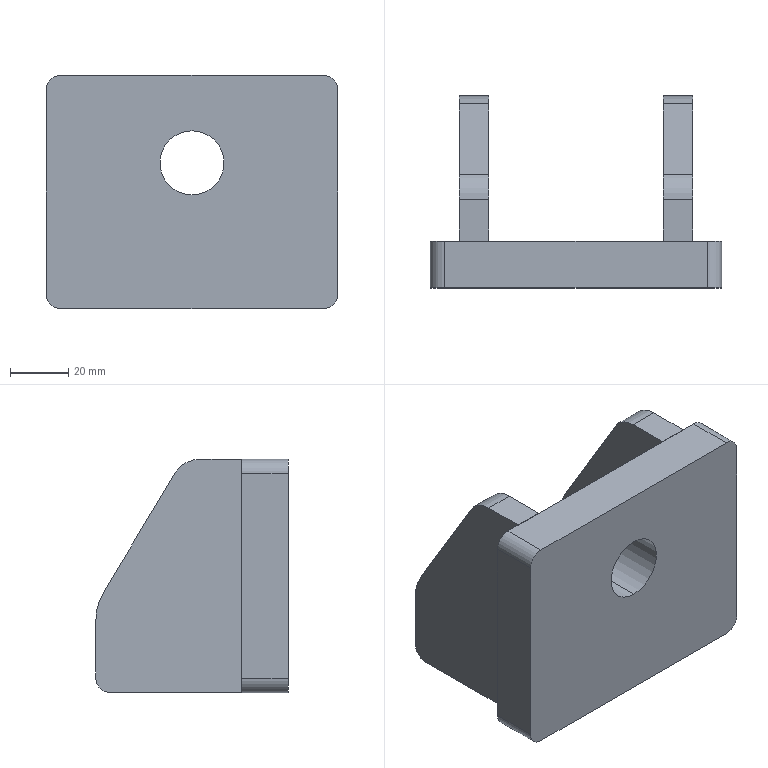Part | SolidWorks | features BaseBody 3 | 3 solids | 32 faces | box 100 x 66 x 80 mm | volume 186311 mm3 | plane 20 | cylinder 12 | commonest cylinder face diameters 10 x6 20 x2 22 x2 40 x2
STEP:
#1=CARTESIAN_POINT('',(30.,8.,30.));
#2=VERTEX_POINT('',#1);
#3=CARTESIAN_POINT('',(30.,8.,-50.));
#4=VERTEX_POINT('',#3);
#5=CARTESIAN_POINT('',(30.,8.,-50.));
#6=DIRECTION('',(0.,0.,-1.));
#7=VECTOR('',#6,1000.);
#8=LINE('',#5,#7);
#9=EDGE_CURVE('',#2,#4,#8,.T.);
#10=ORIENTED_EDGE('',*,*,#9,.T.);
#11=CARTESIAN_POINT('',(40.,8.,-50.));
#12=VERTEX_POINT('',#11);
#13=CARTESIAN_POINT('',(40.,8.,-50.));
#14=DIRECTION('',(-1.,0.,0.));
#15=VECTOR('',#14,1000.);
#16=LINE('',#13,#15);
#17=EDGE_CURVE('',#12,#4,#16,.T.);
#18=ORIENTED_EDGE('',*,*,#17,.F.);
#19=CARTESIAN_POINT('',(40.,8.,30.));
#20=VERTEX_POINT('',#19);
#21=CARTESIAN_POINT('',(40.,8.,-50.));
#22=DIRECTION('',(0.,0.,-1.));
#23=VECTOR('',#22,1000.);
#24=LINE('',#21,#23);
#25=EDGE_CURVE('',#20,#12,#24,.T.);
#26=ORIENTED_EDGE('',*,*,#25,.F.);
#27=CARTESIAN_POINT('',(40.,8.,30.));
#28=DIRECTION('',(-1.,0.,0.));
#29=VECTOR('',#28,1000.);
#30=LINE('',#27,#29);
#31=EDGE_CURVE('',#20,#2,#30,.T.);
#32=ORIENTED_EDGE('',*,*,#31,.T.);
#33=EDGE_LOOP('',(#10,#18,#26,#32));
#34=FACE_OUTER_BOUND('',#33,.T.);
#35=CARTESIAN_POINT('',(40.,8.,-50.));
#36=DIRECTION('',(0.,1.,0.));
#37=DIRECTION('',(0.,0.,1.));
#38=AXIS2_PLACEMENT_3D('',#35,#36,#37);
#39=PLANE('',#38);
#40=ADVANCED_FACE('',(#34),#39,.F.);
#41=CARTESIAN_POINT('',(30.,53.,-50.));
#42=VERTEX_POINT('',#41);
#43=CARTESIAN_POINT('',(30.,53.,-50.));
#44=DIRECTION('',(0.,1.,0.));
#45=VECTOR('',#44,1000.);
#46=LINE('',#43,#45);
#47=EDGE_CURVE('',#4,#42,#46,.T.);
#48=ORIENTED_EDGE('',*,*,#47,.T.);
#49=CARTESIAN_POINT('',(40.,53.,-50.));
#50=VERTEX_POINT('',#49);
#51=CARTESIAN_POINT('',(40.,53.,-50.));
#52=DIRECTION('',(-1.,0.,0.));
#53=VECTOR('',#52,1000.);
#54=LINE('',#51,#53);
#55=EDGE_CURVE('',#50,#42,#54,.T.);
#56=ORIENTED_EDGE('',*,*,#55,.F.);
#57=CARTESIAN_POINT('',(40.,53.,-50.));
#58=DIRECTION('',(0.,1.,0.));
#59=VECTOR('',#58,1000.);
#60=LINE('',#57,#59);
#61=EDGE_CURVE('',#12,#50,#60,.T.);
#62=ORIENTED_EDGE('',*,*,#61,.F.);
#63=ORIENTED_EDGE('',*,*,#17,.T.);
#64=EDGE_LOOP('',(#48,#56,#62,#63));
#65=FACE_OUTER_BOUND('',#64,.T.);
#66=CARTESIAN_POINT('',(40.,53.,-50.));
#67=DIRECTION('',(0.,0.,1.));
#68=DIRECTION('',(0.,-1.,0.));
#69=AXIS2_PLACEMENT_3D('',#66,#67,#68);
#70=PLANE('',#69);
#71=ADVANCED_FACE('',(#65),#70,.F.);
#72=CARTESIAN_POINT('',(30.,58.,-45.));
#73=VERTEX_POINT('',#72);
#74=CARTESIAN_POINT('',(30.,53.,-45.));
#75=DIRECTION('',(1.,0.,0.));
#76=DIRECTION('',(0.,0.,1.));
#77=AXIS2_PLACEMENT_3D('',#74,#75,#76);
#78=CIRCLE('',#77,5.);
#79=EDGE_CURVE('',#42,#73,#78,.T.);
#80=ORIENTED_EDGE('',*,*,#79,.T.);
#81=CARTESIAN_POINT('',(40.,58.,-45.));
#82=VERTEX_POINT('',#81);
#83=CARTESIAN_POINT('',(40.,58.,-45.));
#84=DIRECTION('',(-1.,0.,0.));
#85=VECTOR('',#84,1000.);
#86=LINE('',#83,#85);
#87=EDGE_CURVE('',#82,#73,#86,.T.);
#88=ORIENTED_EDGE('',*,*,#87,.F.);
#89=CARTESIAN_POINT('',(40.,53.,-45.));
#90=DIRECTION('',(1.,0.,0.));
#91=DIRECTION('',(0.,0.,1.));
#92=AXIS2_PLACEMENT_3D('',#89,#90,#91);
#93=CIRCLE('',#92,5.);
#94=EDGE_CURVE('',#50,#82,#93,.T.);
#95=ORIENTED_EDGE('',*,*,#94,.F.);
#96=ORIENTED_EDGE('',*,*,#55,.T.);
#97=EDGE_LOOP('',(#80,#88,#95,#96));
#98=FACE_OUTER_BOUND('',#97,.T.);
#99=CARTESIAN_POINT('',(40.,53.,-45.));
#100=DIRECTION('',(-1.,0.,0.));
#101=DIRECTION('',(0.,0.,1.));
#102=AXIS2_PLACEMENT_3D('',#99,#100,#101);
#103=CYLINDRICAL_SURFACE('',#102,5.);
#104=ADVANCED_FACE('',(#98),#103,.T.);
#105=CARTESIAN_POINT('',(30.,58.,-25.54));
#106=VERTEX_POINT('',#105);
#107=CARTESIAN_POINT('',(30.,58.,-25.54));
#108=DIRECTION('',(0.,0.,1.));
#109=VECTOR('',#108,1000.);
#110=LINE('',#107,#109);
#111=EDGE_CURVE('',#73,#106,#110,.T.);
#112=ORIENTED_EDGE('',*,*,#111,.T.);
#113=CARTESIAN_POINT('',(40.,58.,-25.54));
#114=VERTEX_POINT('',#113);
#115=CARTESIAN_POINT('',(40.,58.,-25.54));
#116=DIRECTION('',(-1.,0.,0.));
#117=VECTOR('',#116,1000.);
#118=LINE('',#115,#117);
#119=EDGE_CURVE('',#114,#106,#118,.T.);
#120=ORIENTED_EDGE('',*,*,#119,.F.);
#121=CARTESIAN_POINT('',(40.,58.,-25.54));
#122=DIRECTION('',(0.,0.,1.));
#123=VECTOR('',#122,1000.);
#124=LINE('',#121,#123);
#125=EDGE_CURVE('',#82,#114,#124,.T.);
#126=ORIENTED_EDGE('',*,*,#125,.F.);
#127=ORIENTED_EDGE('',*,*,#87,.T.);
#128=EDGE_LOOP('',(#112,#120,#126,#127));
#129=FACE_OUTER_BOUND('',#128,.T.);
#130=CARTESIAN_POINT('',(40.,58.,-25.54));
#131=DIRECTION('',(0.,-1.,0.));
#132=DIRECTION('',(0.,0.,-1.));
#133=AXIS2_PLACEMENT_3D('',#130,#131,#132);
#134=PLANE('',#133);
#135=ADVANCED_FACE('',(#129),#134,.F.);
#136=CARTESIAN_POINT('',(30.,55.15,-15.25));
#137=VERTEX_POINT('',#136);
#138=CARTESIAN_POINT('',(30.,38.,-25.54));
#139=DIRECTION('',(1.,0.,0.));
#140=DIRECTION('',(0.,0.,1.));
#141=AXIS2_PLACEMENT_3D('',#138,#139,#140);
#142=CIRCLE('',#141,20.);
#143=EDGE_CURVE('',#106,#137,#142,.T.);
#144=ORIENTED_EDGE('',*,*,#143,.T.);
#145=CARTESIAN_POINT('',(40.,55.15,-15.25));
#146=VERTEX_POINT('',#145);
#147=CARTESIAN_POINT('',(40.,55.15,-15.25));
#148=DIRECTION('',(-1.,0.,0.));
#149=VECTOR('',#148,1000.);
#150=LINE('',#147,#149);
#151=EDGE_CURVE('',#146,#137,#150,.T.);
#152=ORIENTED_EDGE('',*,*,#151,.F.);
#153=CARTESIAN_POINT('',(40.,38.,-25.54));
#154=DIRECTION('',(1.,0.,0.));
#155=DIRECTION('',(0.,0.,1.));
#156=AXIS2_PLACEMENT_3D('',#153,#154,#155);
#157=CIRCLE('',#156,20.);
#158=EDGE_CURVE('',#114,#146,#157,.T.);
#159=ORIENTED_EDGE('',*,*,#158,.F.);
#160=ORIENTED_EDGE('',*,*,#119,.T.);
#161=EDGE_LOOP('',(#144,#152,#159,#160));
#162=FACE_OUTER_BOUND('',#161,.T.);
#163=CARTESIAN_POINT('',(40.,38.,-25.54));
#164=DIRECTION('',(-1.,0.,0.));
#165=DIRECTION('',(0.,0.,1.));
#166=AXIS2_PLACEMENT_3D('',#163,#164,#165);
#167=CYLINDRICAL_SURFACE('',#166,20.);
#168=ADVANCED_FACE('',(#162),#167,.T.);
#169=CARTESIAN_POINT('',(30.,30.913,25.145));
#170=VERTEX_POINT('',#169);
#171=CARTESIAN_POINT('',(30.,30.913,25.145));
#172=DIRECTION('',(0.,-0.5145,0.8575));
#173=VECTOR('',#172,1000.);
#174=LINE('',#171,#173);
#175=EDGE_CURVE('',#137,#170,#174,.T.);
#176=ORIENTED_EDGE('',*,*,#175,.T.);
#177=CARTESIAN_POINT('',(40.,30.913,25.145));
#178=VERTEX_POINT('',#177);
#179=CARTESIAN_POINT('',(40.,30.913,25.145));
#180=DIRECTION('',(-1.,0.,0.));
#181=VECTOR('',#180,1000.);
#182=LINE('',#179,#181);
#183=EDGE_CURVE('',#178,#170,#182,.T.);
#184=ORIENTED_EDGE('',*,*,#183,.F.);
#185=CARTESIAN_POINT('',(40.,30.913,25.145));
#186=DIRECTION('',(0.,-0.5145,0.8575));
#187=VECTOR('',#186,1000.);
#188=LINE('',#185,#187);
#189=EDGE_CURVE('',#146,#178,#188,.T.);
#190=ORIENTED_EDGE('',*,*,#189,.F.);
#191=ORIENTED_EDGE('',*,*,#151,.T.);
#192=EDGE_LOOP('',(#176,#184,#190,#191));
#193=FACE_OUTER_BOUND('',#192,.T.);
#194=CARTESIAN_POINT('',(40.,30.913,25.145));
#195=DIRECTION('',(0.,-0.8575,-0.5145));
#196=DIRECTION('',(0.,0.5145,-0.8575));
#197=AXIS2_PLACEMENT_3D('',#194,#195,#196);
#198=PLANE('',#197);
#199=ADVANCED_FACE('',(#193),#198,.F.);
#200=CARTESIAN_POINT('',(30.,22.338,30.));
#201=VERTEX_POINT('',#200);
#202=CARTESIAN_POINT('',(30.,22.338,20.));
#203=DIRECTION('',(1.,0.,0.));
#204=DIRECTION('',(0.,0.,1.));
#205=AXIS2_PLACEMENT_3D('',#202,#203,#204);
#206=CIRCLE('',#205,10.);
#207=EDGE_CURVE('',#170,#201,#206,.T.);
#208=ORIENTED_EDGE('',*,*,#207,.T.);
#209=CARTESIAN_POINT('',(40.,22.338,30.));
#210=VERTEX_POINT('',#209);
#211=CARTESIAN_POINT('',(40.,22.338,30.));
#212=DIRECTION('',(-1.,0.,0.));
#213=VECTOR('',#212,1000.);
#214=LINE('',#211,#213);
#215=EDGE_CURVE('',#210,#201,#214,.T.);
#216=ORIENTED_EDGE('',*,*,#215,.F.);
#217=CARTESIAN_POINT('',(40.,22.338,20.));
#218=DIRECTION('',(1.,0.,0.));
#219=DIRECTION('',(0.,0.,1.));
#220=AXIS2_PLACEMENT_3D('',#217,#218,#219);
#221=CIRCLE('',#220,10.);
#222=EDGE_CURVE('',#178,#210,#221,.T.);
#223=ORIENTED_EDGE('',*,*,#222,.F.);
#224=ORIENTED_EDGE('',*,*,#183,.T.);
#225=EDGE_LOOP('',(#208,#216,#223,#224));
#226=FACE_OUTER_BOUND('',#225,.T.);
#227=CARTESIAN_POINT('',(40.,22.338,20.));
#228=DIRECTION('',(-1.,0.,0.));
#229=DIRECTION('',(0.,0.,1.));
#230=AXIS2_PLACEMENT_3D('',#227,#228,#229);
#231=CYLINDRICAL_SURFACE('',#230,10.);
#232=ADVANCED_FACE('',(#226),#231,.T.);
#233=CARTESIAN_POINT('',(30.,8.,30.));
#234=DIRECTION('',(0.,-1.,0.));
#235=VECTOR('',#234,1000.);
#236=LINE('',#233,#235);
#237=EDGE_CURVE('',#201,#2,#236,.T.);
#238=ORIENTED_EDGE('',*,*,#237,.T.);
#239=ORIENTED_EDGE('',*,*,#31,.F.);
#240=CARTESIAN_POINT('',(40.,8.,30.));
#241=DIRECTION('',(0.,-1.,0.));
#242=VECTOR('',#241,1000.);
#243=LINE('',#240,#242);
#244=EDGE_CURVE('',#210,#20,#243,.T.);
#245=ORIENTED_EDGE('',*,*,#244,.F.);
#246=ORIENTED_EDGE('',*,*,#215,.T.);
#247=EDGE_LOOP('',(#238,#239,#245,#246));
#248=FACE_OUTER_BOUND('',#247,.T.);
#249=CARTESIAN_POINT('',(40.,8.,30.));
#250=DIRECTION('',(0.,0.,-1.));
#251=DIRECTION('',(-1.,0.,0.));
#252=AXIS2_PLACEMENT_3D('',#249,#250,#251);
#253=PLANE('',#252);
#254=ADVANCED_FACE('',(#248),#253,.F.);
#255=ORIENTED_EDGE('',*,*,#25,.T.);
#256=ORIENTED_EDGE('',*,*,#61,.T.);
#257=ORIENTED_EDGE('',*,*,#94,.T.);
#258=ORIENTED_EDGE('',*,*,#125,.T.);
#259=ORIENTED_EDGE('',*,*,#158,.T.);
#260=ORIENTED_EDGE('',*,*,#189,.T.);
#261=ORIENTED_EDGE('',*,*,#222,.T.);
#262=ORIENTED_EDGE('',*,*,#244,.T.);
#263=EDGE_LOOP('',(#255,#256,#257,#258,#259,#260,#261,#262));
#264=FACE_OUTER_BOUND('',#263,.T.);
#265=CARTESIAN_POINT('',(40.,22.338,20.));
#266=DIRECTION('',(-1.,0.,0.));
#267=DIRECTION('',(0.,0.,1.));
#268=AXIS2_PLACEMENT_3D('',#265,#266,#267);
#269=PLANE('',#268);
#270=ADVANCED_FACE('',(#264),#269,.F.);
#271=ORIENTED_EDGE('',*,*,#9,.F.);
#272=ORIENTED_EDGE('',*,*,#237,.F.);
#273=ORIENTED_EDGE('',*,*,#207,.F.);
#274=ORIENTED_EDGE('',*,*,#175,.F.);
#275=ORIENTED_EDGE('',*,*,#143,.F.);
#276=ORIENTED_EDGE('',*,*,#111,.F.);
#277=ORIENTED_EDGE('',*,*,#79,.F.);
#278=ORIENTED_EDGE('',*,*,#47,.F.);
#279=EDGE_LOOP('',(#271,#272,#273,#274,#275,#276,#277,#278));
#280=FACE_OUTER_BOUND('',#279,.T.);
#281=CARTESIAN_POINT('',(30.,22.338,20.));
#282=DIRECTION('',(-1.,0.,0.));
#283=DIRECTION('',(0.,0.,1.));
#284=AXIS2_PLACEMENT_3D('',#281,#282,#283);
#285=PLANE('',#284);
#286=ADVANCED_FACE('',(#280),#285,.T.);
#287=CLOSED_SHELL('',(#40,#71,#104,#135,#168,#199,#232,#254,#270,#286));
#288=MANIFOLD_SOLID_BREP('',#287);
#289=CARTESIAN_POINT('',(-30.,8.,30.));
#290=VERTEX_POINT('',#289);
#291=CARTESIAN_POINT('',(-30.,8.,-50.));
#292=VERTEX_POINT('',#291);
#293=CARTESIAN_POINT('',(-30.,8.,-50.));
#294=DIRECTION('',(0.,0.,-1.));
#295=VECTOR('',#294,1000.);
#296=LINE('',#293,#295);
#297=EDGE_CURVE('',#290,#292,#296,.T.);
#298=ORIENTED_EDGE('',*,*,#297,.F.);
#299=CARTESIAN_POINT('',(-40.,8.,30.));
#300=VERTEX_POINT('',#299);
#301=CARTESIAN_POINT('',(-40.,8.,30.));
#302=DIRECTION('',(1.,0.,0.));
#303=VECTOR('',#302,1000.);
#304=LINE('',#301,#303);
#305=EDGE_CURVE('',#300,#290,#304,.T.);
#306=ORIENTED_EDGE('',*,*,#305,.F.);
#307=CARTESIAN_POINT('',(-40.,8.,-50.));
#308=VERTEX_POINT('',#307);
#309=CARTESIAN_POINT('',(-40.,8.,-50.));
#310=DIRECTION('',(0.,0.,-1.));
#311=VECTOR('',#310,1000.);
#312=LINE('',#309,#311);
#313=EDGE_CURVE('',#300,#308,#312,.T.);
#314=ORIENTED_EDGE('',*,*,#313,.T.);
#315=CARTESIAN_POINT('',(-40.,8.,-50.));
#316=DIRECTION('',(1.,0.,0.));
#317=VECTOR('',#316,1000.);
#318=LINE('',#315,#317);
#319=EDGE_CURVE('',#308,#292,#318,.T.);
#320=ORIENTED_EDGE('',*,*,#319,.T.);
#321=EDGE_LOOP('',(#298,#306,#314,#320));
#322=FACE_OUTER_BOUND('',#321,.T.);
#323=CARTESIAN_POINT('',(-40.,8.,-50.));
#324=DIRECTION('',(0.,1.,0.));
#325=DIRECTION('',(0.,0.,1.));
#326=AXIS2_PLACEMENT_3D('',#323,#324,#325);
#327=PLANE('',#326);
#328=ADVANCED_FACE('',(#322),#327,.F.);
#329=CARTESIAN_POINT('',(-30.,53.,-50.));
#330=VERTEX_POINT('',#329);
#331=CARTESIAN_POINT('',(-30.,53.,-50.));
#332=DIRECTION('',(0.,1.,0.));
#333=VECTOR('',#332,1000.);
#334=LINE('',#331,#333);
#335=EDGE_CURVE('',#292,#330,#334,.T.);
#336=ORIENTED_EDGE('',*,*,#335,.F.);
#337=ORIENTED_EDGE('',*,*,#319,.F.);
#338=CARTESIAN_POINT('',(-40.,53.,-50.));
#339=VERTEX_POINT('',#338);
#340=CARTESIAN_POINT('',(-40.,53.,-50.));
#341=DIRECTION('',(0.,1.,0.));
#342=VECTOR('',#341,1000.);
#343=LINE('',#340,#342);
#344=EDGE_CURVE('',#308,#339,#343,.T.);
#345=ORIENTED_EDGE('',*,*,#344,.T.);
#346=CARTESIAN_POINT('',(-40.,53.,-50.));
#347=DIRECTION('',(1.,0.,0.));
#348=VECTOR('',#347,1000.);
#349=LINE('',#346,#348);
#350=EDGE_CURVE('',#339,#330,#349,.T.);
#351=ORIENTED_EDGE('',*,*,#350,.T.);
#352=EDGE_LOOP('',(#336,#337,#345,#351));
#353=FACE_OUTER_BOUND('',#352,.T.);
#354=CARTESIAN_POINT('',(-40.,53.,-50.));
#355=DIRECTION('',(0.,0.,1.));
#356=DIRECTION('',(0.,-1.,0.));
#357=AXIS2_PLACEMENT_3D('',#354,#355,#356);
#358=PLANE('',#357);
#359=ADVANCED_FACE('',(#353),#358,.F.);
#360=CARTESIAN_POINT('',(-30.,58.,-45.));
#361=VERTEX_POINT('',#360);
#362=CARTESIAN_POINT('',(-30.,53.,-45.));
#363=DIRECTION('',(1.,0.,0.));
#364=DIRECTION('',(0.,0.,1.));
#365=AXIS2_PLACEMENT_3D('',#362,#363,#364);
#366=CIRCLE('',#365,5.);
#367=EDGE_CURVE('',#330,#361,#366,.T.);
#368=ORIENTED_EDGE('',*,*,#367,.F.);
#369=ORIENTED_EDGE('',*,*,#350,.F.);
#370=CARTESIAN_POINT('',(-40.,58.,-45.));
#371=VERTEX_POINT('',#370);
#372=CARTESIAN_POINT('',(-40.,53.,-45.));
#373=DIRECTION('',(1.,0.,0.));
#374=DIRECTION('',(0.,0.,1.));
#375=AXIS2_PLACEMENT_3D('',#372,#373,#374);
#376=CIRCLE('',#375,5.);
#377=EDGE_CURVE('',#339,#371,#376,.T.);
#378=ORIENTED_EDGE('',*,*,#377,.T.);
#379=CARTESIAN_POINT('',(-40.,58.,-45.));
#380=DIRECTION('',(1.,0.,0.));
#381=VECTOR('',#380,1000.);
#382=LINE('',#379,#381);
#383=EDGE_CURVE('',#371,#361,#382,.T.);
#384=ORIENTED_EDGE('',*,*,#383,.T.);
#385=EDGE_LOOP('',(#368,#369,#378,#384));
#386=FACE_OUTER_BOUND('',#385,.T.);
#387=CARTESIAN_POINT('',(-40.,53.,-45.));
#388=DIRECTION('',(1.,0.,0.));
#389=DIRECTION('',(0.,0.,1.));
#390=AXIS2_PLACEMENT_3D('',#387,#388,#389);
#391=CYLINDRICAL_SURFACE('',#390,5.);
#392=ADVANCED_FACE('',(#386),#391,.T.);
#393=CARTESIAN_POINT('',(-30.,58.,-25.54));
#394=VERTEX_POINT('',#393);
#395=CARTESIAN_POINT('',(-30.,58.,-25.54));
#396=DIRECTION('',(0.,0.,1.));
#397=VECTOR('',#396,1000.);
#398=LINE('',#395,#397);
#399=EDGE_CURVE('',#361,#394,#398,.T.);
#400=ORIENTED_EDGE('',*,*,#399,.F.);
#401=ORIENTED_EDGE('',*,*,#383,.F.);
#402=CARTESIAN_POINT('',(-40.,58.,-25.54));
#403=VERTEX_POINT('',#402);
#404=CARTESIAN_POINT('',(-40.,58.,-25.54));
#405=DIRECTION('',(0.,0.,1.));
#406=VECTOR('',#405,1000.);
#407=LINE('',#404,#406);
#408=EDGE_CURVE('',#371,#403,#407,.T.);
#409=ORIENTED_EDGE('',*,*,#408,.T.);
#410=CARTESIAN_POINT('',(-40.,58.,-25.54));
#411=DIRECTION('',(1.,0.,0.));
#412=VECTOR('',#411,1000.);
#413=LINE('',#410,#412);
#414=EDGE_CURVE('',#403,#394,#413,.T.);
#415=ORIENTED_EDGE('',*,*,#414,.T.);
#416=EDGE_LOOP('',(#400,#401,#409,#415));
#417=FACE_OUTER_BOUND('',#416,.T.);
#418=CARTESIAN_POINT('',(-40.,58.,-25.54));
#419=DIRECTION('',(0.,-1.,0.));
#420=DIRECTION('',(0.,0.,-1.));
#421=AXIS2_PLACEMENT_3D('',#418,#419,#420);
#422=PLANE('',#421);
#423=ADVANCED_FACE('',(#417),#422,.F.);
#424=CARTESIAN_POINT('',(-30.,55.15,-15.25));
#425=VERTEX_POINT('',#424);
#426=CARTESIAN_POINT('',(-30.,38.,-25.54));
#427=DIRECTION('',(1.,0.,0.));
#428=DIRECTION('',(0.,0.,1.));
#429=AXIS2_PLACEMENT_3D('',#426,#427,#428);
#430=CIRCLE('',#429,20.);
#431=EDGE_CURVE('',#394,#425,#430,.T.);
#432=ORIENTED_EDGE('',*,*,#431,.F.);
#433=ORIENTED_EDGE('',*,*,#414,.F.);
#434=CARTESIAN_POINT('',(-40.,55.15,-15.25));
#435=VERTEX_POINT('',#434);
#436=CARTESIAN_POINT('',(-40.,38.,-25.54));
#437=DIRECTION('',(1.,0.,0.));
#438=DIRECTION('',(0.,0.,1.));
#439=AXIS2_PLACEMENT_3D('',#436,#437,#438);
#440=CIRCLE('',#439,20.);
#441=EDGE_CURVE('',#403,#435,#440,.T.);
#442=ORIENTED_EDGE('',*,*,#441,.T.);
#443=CARTESIAN_POINT('',(-40.,55.15,-15.25));
#444=DIRECTION('',(1.,0.,0.));
#445=VECTOR('',#444,1000.);
#446=LINE('',#443,#445);
#447=EDGE_CURVE('',#435,#425,#446,.T.);
#448=ORIENTED_EDGE('',*,*,#447,.T.);
#449=EDGE_LOOP('',(#432,#433,#442,#448));
#450=FACE_OUTER_BOUND('',#449,.T.);
#451=CARTESIAN_POINT('',(-40.,38.,-25.54));
#452=DIRECTION('',(1.,0.,0.));
#453=DIRECTION('',(0.,0.,1.));
#454=AXIS2_PLACEMENT_3D('',#451,#452,#453);
#455=CYLINDRICAL_SURFACE('',#454,20.);
#456=ADVANCED_FACE('',(#450),#455,.T.);
#457=CARTESIAN_POINT('',(-30.,30.913,25.145));
#458=VERTEX_POINT('',#457);
#459=CARTESIAN_POINT('',(-30.,30.913,25.145));
#460=DIRECTION('',(0.,-0.5145,0.8575));
#461=VECTOR('',#460,1000.);
#462=LINE('',#459,#461);
#463=EDGE_CURVE('',#425,#458,#462,.T.);
#464=ORIENTED_EDGE('',*,*,#463,.F.);
#465=ORIENTED_EDGE('',*,*,#447,.F.);
#466=CARTESIAN_POINT('',(-40.,30.913,25.145));
#467=VERTEX_POINT('',#466);
#468=CARTESIAN_POINT('',(-40.,30.913,25.145));
#469=DIRECTION('',(0.,-0.5145,0.8575));
#470=VECTOR('',#469,1000.);
#471=LINE('',#468,#470);
#472=EDGE_CURVE('',#435,#467,#471,.T.);
#473=ORIENTED_EDGE('',*,*,#472,.T.);
#474=CARTESIAN_POINT('',(-40.,30.913,25.145));
#475=DIRECTION('',(1.,0.,0.));
#476=VECTOR('',#475,1000.);
#477=LINE('',#474,#476);
#478=EDGE_CURVE('',#467,#458,#477,.T.);
#479=ORIENTED_EDGE('',*,*,#478,.T.);
#480=EDGE_LOOP('',(#464,#465,#473,#479));
#481=FACE_OUTER_BOUND('',#480,.T.);
#482=CARTESIAN_POINT('',(-40.,30.913,25.145));
#483=DIRECTION('',(0.,-0.8575,-0.5145));
#484=DIRECTION('',(0.,0.5145,-0.8575));
#485=AXIS2_PLACEMENT_3D('',#482,#483,#484);
#486=PLANE('',#485);
#487=ADVANCED_FACE('',(#481),#486,.F.);
#488=CARTESIAN_POINT('',(-30.,22.338,30.));
#489=VERTEX_POINT('',#488);
#490=CARTESIAN_POINT('',(-30.,22.338,20.));
#491=DIRECTION('',(1.,0.,0.));
#492=DIRECTION('',(0.,0.,1.));
#493=AXIS2_PLACEMENT_3D('',#490,#491,#492);
#494=CIRCLE('',#493,10.);
#495=EDGE_CURVE('',#458,#489,#494,.T.);
#496=ORIENTED_EDGE('',*,*,#495,.F.);
#497=ORIENTED_EDGE('',*,*,#478,.F.);
#498=CARTESIAN_POINT('',(-40.,22.338,30.));
#499=VERTEX_POINT('',#498);
#500=CARTESIAN_POINT('',(-40.,22.338,20.));
#501=DIRECTION('',(1.,0.,0.));
#502=DIRECTION('',(0.,0.,1.));
#503=AXIS2_PLACEMENT_3D('',#500,#501,#502);
#504=CIRCLE('',#503,10.);
#505=EDGE_CURVE('',#467,#499,#504,.T.);
#506=ORIENTED_EDGE('',*,*,#505,.T.);
#507=CARTESIAN_POINT('',(-40.,22.338,30.));
#508=DIRECTION('',(1.,0.,0.));
#509=VECTOR('',#508,1000.);
#510=LINE('',#507,#509);
#511=EDGE_CURVE('',#499,#489,#510,.T.);
#512=ORIENTED_EDGE('',*,*,#511,.T.);
#513=EDGE_LOOP('',(#496,#497,#506,#512));
#514=FACE_OUTER_BOUND('',#513,.T.);
#515=CARTESIAN_POINT('',(-40.,22.338,20.));
#516=DIRECTION('',(1.,0.,0.));
#517=DIRECTION('',(0.,0.,1.));
#518=AXIS2_PLACEMENT_3D('',#515,#516,#517);
#519=CYLINDRICAL_SURFACE('',#518,10.);
#520=ADVANCED_FACE('',(#514),#519,.T.);
#521=CARTESIAN_POINT('',(-30.,8.,30.));
#522=DIRECTION('',(0.,-1.,0.));
#523=VECTOR('',#522,1000.);
#524=LINE('',#521,#523);
#525=EDGE_CURVE('',#489,#290,#524,.T.);
#526=ORIENTED_EDGE('',*,*,#525,.F.);
#527=ORIENTED_EDGE('',*,*,#511,.F.);
#528=CARTESIAN_POINT('',(-40.,8.,30.));
#529=DIRECTION('',(0.,-1.,0.));
#530=VECTOR('',#529,1000.);
#531=LINE('',#528,#530);
#532=EDGE_CURVE('',#499,#300,#531,.T.);
#533=ORIENTED_EDGE('',*,*,#532,.T.);
#534=ORIENTED_EDGE('',*,*,#305,.T.);
#535=EDGE_LOOP('',(#526,#527,#533,#534));
#536=FACE_OUTER_BOUND('',#535,.T.);
#537=CARTESIAN_POINT('',(-40.,8.,30.));
#538=DIRECTION('',(0.,0.,-1.));
#539=DIRECTION('',(1.,0.,0.));
#540=AXIS2_PLACEMENT_3D('',#537,#538,#539);
#541=PLANE('',#540);
#542=ADVANCED_FACE('',(#536),#541,.F.);
#543=ORIENTED_EDGE('',*,*,#313,.F.);
#544=ORIENTED_EDGE('',*,*,#532,.F.);
#545=ORIENTED_EDGE('',*,*,#505,.F.);
#546=ORIENTED_EDGE('',*,*,#472,.F.);
#547=ORIENTED_EDGE('',*,*,#441,.F.);
#548=ORIENTED_EDGE('',*,*,#408,.F.);
#549=ORIENTED_EDGE('',*,*,#377,.F.);
#550=ORIENTED_EDGE('',*,*,#344,.F.);
#551=EDGE_LOOP('',(#543,#544,#545,#546,#547,#548,#549,#550));
#552=FACE_OUTER_BOUND('',#551,.T.);
#553=CARTESIAN_POINT('',(-40.,22.338,20.));
#554=DIRECTION('',(1.,0.,0.));
#555=DIRECTION('',(0.,0.,1.));
#556=AXIS2_PLACEMENT_3D('',#553,#554,#555);
#557=PLANE('',#556);
#558=ADVANCED_FACE('',(#552),#557,.F.);
#559=ORIENTED_EDGE('',*,*,#297,.T.);
#560=ORIENTED_EDGE('',*,*,#335,.T.);
#561=ORIENTED_EDGE('',*,*,#367,.T.);
#562=ORIENTED_EDGE('',*,*,#399,.T.);
#563=ORIENTED_EDGE('',*,*,#431,.T.);
#564=ORIENTED_EDGE('',*,*,#463,.T.);
#565=ORIENTED_EDGE('',*,*,#495,.T.);
#566=ORIENTED_EDGE('',*,*,#525,.T.);
#567=EDGE_LOOP('',(#559,#560,#561,#562,#563,#564,#565,#566));
#568=FACE_OUTER_BOUND('',#567,.T.);
#569=CARTESIAN_POINT('',(-30.,22.338,20.));
#570=DIRECTION('',(1.,0.,0.));
#571=DIRECTION('',(0.,0.,1.));
#572=AXIS2_PLACEMENT_3D('',#569,#570,#571);
#573=PLANE('',#572);
#574=ADVANCED_FACE('',(#568),#573,.T.);
#575=CLOSED_SHELL('',(#328,#359,#392,#423,#456,#487,#520,#542,#558,#574));
#576=MANIFOLD_SOLID_BREP('',#575);
#577=CARTESIAN_POINT('',(0.,8.,-11.));
#578=VERTEX_POINT('',#577);
#579=CARTESIAN_POINT('',(0.,8.,11.));
#580=VERTEX_POINT('',#579);
#581=CARTESIAN_POINT('',(0.,8.,0.));
#582=DIRECTION('',(0.,1.,0.));
#583=DIRECTION('',(0.,0.,1.));
#584=AXIS2_PLACEMENT_3D('',#581,#582,#583);
#585=CIRCLE('',#584,11.);
#586=EDGE_CURVE('',#578,#580,#585,.T.);
#587=ORIENTED_EDGE('',*,*,#586,.T.);
#588=CARTESIAN_POINT('',(0.,-8.,11.));
#589=VERTEX_POINT('',#588);
#590=CARTESIAN_POINT('',(0.,8.,11.));
#591=DIRECTION('',(0.,-1.,0.));
#592=VECTOR('',#591,1000.);
#593=LINE('',#590,#592);
#594=EDGE_CURVE('',#580,#589,#593,.T.);
#595=ORIENTED_EDGE('',*,*,#594,.T.);
#596=CARTESIAN_POINT('',(0.,-8.,-11.));
#597=VERTEX_POINT('',#596);
#598=CARTESIAN_POINT('',(0.,-8.,0.));
#599=DIRECTION('',(0.,1.,0.));
#600=DIRECTION('',(0.,0.,1.));
#601=AXIS2_PLACEMENT_3D('',#598,#599,#600);
#602=CIRCLE('',#601,11.);
#603=EDGE_CURVE('',#597,#589,#602,.T.);
#604=ORIENTED_EDGE('',*,*,#603,.F.);
#605=CARTESIAN_POINT('',(0.,8.,-11.));
#606=DIRECTION('',(0.,-1.,0.));
#607=VECTOR('',#606,1000.);
#608=LINE('',#605,#607);
#609=EDGE_CURVE('',#578,#597,#608,.T.);
#610=ORIENTED_EDGE('',*,*,#609,.F.);
#611=EDGE_LOOP('',(#587,#595,#604,#610));
#612=FACE_OUTER_BOUND('',#611,.T.);
#613=CARTESIAN_POINT('',(0.,8.,0.));
#614=DIRECTION('',(0.,-1.,0.));
#615=DIRECTION('',(0.,0.,-1.));
#616=AXIS2_PLACEMENT_3D('',#613,#614,#615);
#617=CYLINDRICAL_SURFACE('',#616,11.);
#618=ADVANCED_FACE('',(#612),#617,.F.);
#619=CARTESIAN_POINT('',(-45.,8.,-50.));
#620=VERTEX_POINT('',#619);
#621=CARTESIAN_POINT('',(-50.,8.,-45.));
#622=VERTEX_POINT('',#621);
#623=CARTESIAN_POINT('',(-45.,8.,-45.));
#624=DIRECTION('',(0.,1.,0.));
#625=DIRECTION('',(0.,0.,1.));
#626=AXIS2_PLACEMENT_3D('',#623,#624,#625);
#627=CIRCLE('',#626,5.);
#628=EDGE_CURVE('',#620,#622,#627,.T.);
#629=ORIENTED_EDGE('',*,*,#628,.T.);
#630=CARTESIAN_POINT('',(-50.,8.,25.));
#631=VERTEX_POINT('',#630);
#632=CARTESIAN_POINT('',(-50.,8.,-25.));
#633=DIRECTION('',(0.,0.,1.));
#634=VECTOR('',#633,1000.);
#635=LINE('',#632,#634);
#636=EDGE_CURVE('',#622,#631,#635,.T.);
#637=ORIENTED_EDGE('',*,*,#636,.T.);
#638=CARTESIAN_POINT('',(-45.,8.,30.));
#639=VERTEX_POINT('',#638);
#640=CARTESIAN_POINT('',(-45.,8.,25.));
#641=DIRECTION('',(0.,1.,0.));
#642=DIRECTION('',(0.,0.,1.));
#643=AXIS2_PLACEMENT_3D('',#640,#641,#642);
#644=CIRCLE('',#643,5.);
#645=EDGE_CURVE('',#631,#639,#644,.T.);
#646=ORIENTED_EDGE('',*,*,#645,.T.);
#647=CARTESIAN_POINT('',(45.,8.,30.));
#648=VERTEX_POINT('',#647);
#649=CARTESIAN_POINT('',(-45.,8.,30.));
#650=DIRECTION('',(1.,0.,0.));
#651=VECTOR('',#650,1000.);
#652=LINE('',#649,#651);
#653=EDGE_CURVE('',#639,#648,#652,.T.);
#654=ORIENTED_EDGE('',*,*,#653,.T.);
#655=CARTESIAN_POINT('',(50.,8.,25.));
#656=VERTEX_POINT('',#655);
#657=CARTESIAN_POINT('',(45.,8.,25.));
#658=DIRECTION('',(0.,1.,0.));
#659=DIRECTION('',(0.,0.,1.));
#660=AXIS2_PLACEMENT_3D('',#657,#658,#659);
#661=CIRCLE('',#660,5.);
#662=EDGE_CURVE('',#648,#656,#661,.T.);
#663=ORIENTED_EDGE('',*,*,#662,.T.);
#664=CARTESIAN_POINT('',(50.,8.,-45.));
#665=VERTEX_POINT('',#664);
#666=CARTESIAN_POINT('',(50.,8.,-25.));
#667=DIRECTION('',(0.,0.,-1.));
#668=VECTOR('',#667,1000.);
#669=LINE('',#666,#668);
#670=EDGE_CURVE('',#656,#665,#669,.T.);
#671=ORIENTED_EDGE('',*,*,#670,.T.);
#672=CARTESIAN_POINT('',(45.,8.,-50.));
#673=VERTEX_POINT('',#672);
#674=CARTESIAN_POINT('',(45.,8.,-45.));
#675=DIRECTION('',(0.,1.,0.));
#676=DIRECTION('',(0.,0.,-1.));
#677=AXIS2_PLACEMENT_3D('',#674,#675,#676);
#678=CIRCLE('',#677,5.);
#679=EDGE_CURVE('',#665,#673,#678,.T.);
#680=ORIENTED_EDGE('',*,*,#679,.T.);
#681=CARTESIAN_POINT('',(-45.,8.,-50.));
#682=DIRECTION('',(-1.,0.,0.));
#683=VECTOR('',#682,1000.);
#684=LINE('',#681,#683);
#685=EDGE_CURVE('',#673,#620,#684,.T.);
#686=ORIENTED_EDGE('',*,*,#685,.T.);
#687=EDGE_LOOP('',(#629,#637,#646,#654,#663,#671,#680,#686));
#688=FACE_OUTER_BOUND('',#687,.T.);
#689=ORIENTED_EDGE('',*,*,#586,.F.);
#690=CARTESIAN_POINT('',(0.,8.,0.));
#691=DIRECTION('',(0.,1.,0.));
#692=DIRECTION('',(0.,0.,1.));
#693=AXIS2_PLACEMENT_3D('',#690,#691,#692);
#694=CIRCLE('',#693,11.);
#695=EDGE_CURVE('',#580,#578,#694,.T.);
#696=ORIENTED_EDGE('',*,*,#695,.F.);
#697=EDGE_LOOP('',(#689,#696));
#698=FACE_BOUND('',#697,.T.);
#699=CARTESIAN_POINT('',(-45.,8.,-25.));
#700=DIRECTION('',(0.,1.,0.));
#701=DIRECTION('',(0.,0.,1.));
#702=AXIS2_PLACEMENT_3D('',#699,#700,#701);
#703=PLANE('',#702);
#704=ADVANCED_FACE('',(#688,#698),#703,.T.);
#705=CARTESIAN_POINT('',(-45.,-8.,-50.));
#706=VERTEX_POINT('',#705);
#707=CARTESIAN_POINT('',(-50.,-8.,-45.));
#708=VERTEX_POINT('',#707);
#709=CARTESIAN_POINT('',(-45.,-8.,-45.));
#710=DIRECTION('',(0.,1.,0.));
#711=DIRECTION('',(0.,0.,1.));
#712=AXIS2_PLACEMENT_3D('',#709,#710,#711);
#713=CIRCLE('',#712,5.);
#714=EDGE_CURVE('',#706,#708,#713,.T.);
#715=ORIENTED_EDGE('',*,*,#714,.F.);
#716=CARTESIAN_POINT('',(45.,-8.,-50.));
#717=VERTEX_POINT('',#716);
#718=CARTESIAN_POINT('',(-45.,-8.,-50.));
#719=DIRECTION('',(-1.,0.,0.));
#720=VECTOR('',#719,1000.);
#721=LINE('',#718,#720);
#722=EDGE_CURVE('',#717,#706,#721,.T.);
#723=ORIENTED_EDGE('',*,*,#722,.F.);
#724=CARTESIAN_POINT('',(50.,-8.,-45.));
#725=VERTEX_POINT('',#724);
#726=CARTESIAN_POINT('',(45.,-8.,-45.));
#727=DIRECTION('',(0.,1.,0.));
#728=DIRECTION('',(0.,0.,-1.));
#729=AXIS2_PLACEMENT_3D('',#726,#727,#728);
#730=CIRCLE('',#729,5.);
#731=EDGE_CURVE('',#725,#717,#730,.T.);
#732=ORIENTED_EDGE('',*,*,#731,.F.);
#733=CARTESIAN_POINT('',(50.,-8.,25.));
#734=VERTEX_POINT('',#733);
#735=CARTESIAN_POINT('',(50.,-8.,-25.));
#736=DIRECTION('',(0.,0.,-1.));
#737=VECTOR('',#736,1000.);
#738=LINE('',#735,#737);
#739=EDGE_CURVE('',#734,#725,#738,.T.);
#740=ORIENTED_EDGE('',*,*,#739,.F.);
#741=CARTESIAN_POINT('',(45.,-8.,30.));
#742=VERTEX_POINT('',#741);
#743=CARTESIAN_POINT('',(45.,-8.,25.));
#744=DIRECTION('',(0.,1.,0.));
#745=DIRECTION('',(0.,0.,1.));
#746=AXIS2_PLACEMENT_3D('',#743,#744,#745);
#747=CIRCLE('',#746,5.);
#748=EDGE_CURVE('',#742,#734,#747,.T.);
#749=ORIENTED_EDGE('',*,*,#748,.F.);
#750=CARTESIAN_POINT('',(-45.,-8.,30.));
#751=VERTEX_POINT('',#750);
#752=CARTESIAN_POINT('',(-45.,-8.,30.));
#753=DIRECTION('',(1.,0.,0.));
#754=VECTOR('',#753,1000.);
#755=LINE('',#752,#754);
#756=EDGE_CURVE('',#751,#742,#755,.T.);
#757=ORIENTED_EDGE('',*,*,#756,.F.);
#758=CARTESIAN_POINT('',(-50.,-8.,25.));
#759=VERTEX_POINT('',#758);
#760=CARTESIAN_POINT('',(-45.,-8.,25.));
#761=DIRECTION('',(0.,1.,0.));
#762=DIRECTION('',(0.,0.,1.));
#763=AXIS2_PLACEMENT_3D('',#760,#761,#762);
#764=CIRCLE('',#763,5.);
#765=EDGE_CURVE('',#759,#751,#764,.T.);
#766=ORIENTED_EDGE('',*,*,#765,.F.);
#767=CARTESIAN_POINT('',(-50.,-8.,-25.));
#768=DIRECTION('',(0.,0.,1.));
#769=VECTOR('',#768,1000.);
#770=LINE('',#767,#769);
#771=EDGE_CURVE('',#708,#759,#770,.T.);
#772=ORIENTED_EDGE('',*,*,#771,.F.);
#773=EDGE_LOOP('',(#715,#723,#732,#740,#749,#757,#766,#772));
#774=FACE_OUTER_BOUND('',#773,.T.);
#775=ORIENTED_EDGE('',*,*,#603,.T.);
#776=CARTESIAN_POINT('',(0.,-8.,0.));
#777=DIRECTION('',(0.,1.,0.));
#778=DIRECTION('',(0.,0.,1.));
#779=AXIS2_PLACEMENT_3D('',#776,#777,#778);
#780=CIRCLE('',#779,11.);
#781=EDGE_CURVE('',#589,#597,#780,.T.);
#782=ORIENTED_EDGE('',*,*,#781,.T.);
#783=EDGE_LOOP('',(#775,#782));
#784=FACE_BOUND('',#783,.T.);
#785=CARTESIAN_POINT('',(-45.,-8.,-25.));
#786=DIRECTION('',(0.,1.,0.));
#787=DIRECTION('',(0.,0.,1.));
#788=AXIS2_PLACEMENT_3D('',#785,#786,#787);
#789=PLANE('',#788);
#790=ADVANCED_FACE('',(#774,#784),#789,.F.);
#791=ORIENTED_EDGE('',*,*,#714,.T.);
#792=CARTESIAN_POINT('',(-50.,8.,-45.));
#793=DIRECTION('',(0.,-1.,0.));
#794=VECTOR('',#793,1000.);
#795=LINE('',#792,#794);
#796=EDGE_CURVE('',#622,#708,#795,.T.);
#797=ORIENTED_EDGE('',*,*,#796,.F.);
#798=ORIENTED_EDGE('',*,*,#628,.F.);
#799=CARTESIAN_POINT('',(-45.,8.,-50.));
#800=DIRECTION('',(0.,-1.,0.));
#801=VECTOR('',#800,1000.);
#802=LINE('',#799,#801);
#803=EDGE_CURVE('',#620,#706,#802,.T.);
#804=ORIENTED_EDGE('',*,*,#803,.T.);
#805=EDGE_LOOP('',(#791,#797,#798,#804));
#806=FACE_OUTER_BOUND('',#805,.T.);
#807=CARTESIAN_POINT('',(-45.,8.,-45.));
#808=DIRECTION('',(0.,-1.,0.));
#809=DIRECTION('',(0.,0.,-1.));
#810=AXIS2_PLACEMENT_3D('',#807,#808,#809);
#811=CYLINDRICAL_SURFACE('',#810,5.);
#812=ADVANCED_FACE('',(#806),#811,.T.);
#813=ORIENTED_EDGE('',*,*,#771,.T.);
#814=CARTESIAN_POINT('',(-50.,8.,25.));
#815=DIRECTION('',(0.,-1.,0.));
#816=VECTOR('',#815,1000.);
#817=LINE('',#814,#816);
#818=EDGE_CURVE('',#631,#759,#817,.T.);
#819=ORIENTED_EDGE('',*,*,#818,.F.);
#820=ORIENTED_EDGE('',*,*,#636,.F.);
#821=ORIENTED_EDGE('',*,*,#796,.T.);
#822=EDGE_LOOP('',(#813,#819,#820,#821));
#823=FACE_OUTER_BOUND('',#822,.T.);
#824=CARTESIAN_POINT('',(-50.,8.,-25.));
#825=DIRECTION('',(1.,0.,0.));
#826=DIRECTION('',(0.,0.,-1.));
#827=AXIS2_PLACEMENT_3D('',#824,#825,#826);
#828=PLANE('',#827);
#829=ADVANCED_FACE('',(#823),#828,.F.);
#830=ORIENTED_EDGE('',*,*,#765,.T.);
#831=CARTESIAN_POINT('',(-45.,8.,30.));
#832=DIRECTION('',(0.,-1.,0.));
#833=VECTOR('',#832,1000.);
#834=LINE('',#831,#833);
#835=EDGE_CURVE('',#639,#751,#834,.T.);
#836=ORIENTED_EDGE('',*,*,#835,.F.);
#837=ORIENTED_EDGE('',*,*,#645,.F.);
#838=ORIENTED_EDGE('',*,*,#818,.T.);
#839=EDGE_LOOP('',(#830,#836,#837,#838));
#840=FACE_OUTER_BOUND('',#839,.T.);
#841=CARTESIAN_POINT('',(-45.,8.,25.));
#842=DIRECTION('',(0.,-1.,0.));
#843=DIRECTION('',(0.,0.,-1.));
#844=AXIS2_PLACEMENT_3D('',#841,#842,#843);
#845=CYLINDRICAL_SURFACE('',#844,5.);
#846=ADVANCED_FACE('',(#840),#845,.T.);
#847=ORIENTED_EDGE('',*,*,#756,.T.);
#848=CARTESIAN_POINT('',(45.,8.,30.));
#849=DIRECTION('',(0.,-1.,0.));
#850=VECTOR('',#849,1000.);
#851=LINE('',#848,#850);
#852=EDGE_CURVE('',#648,#742,#851,.T.);
#853=ORIENTED_EDGE('',*,*,#852,.F.);
#854=ORIENTED_EDGE('',*,*,#653,.F.);
#855=ORIENTED_EDGE('',*,*,#835,.T.);
#856=EDGE_LOOP('',(#847,#853,#854,#855));
#857=FACE_OUTER_BOUND('',#856,.T.);
#858=CARTESIAN_POINT('',(-45.,8.,30.));
#859=DIRECTION('',(0.,0.,-1.));
#860=DIRECTION('',(-1.,0.,0.));
#861=AXIS2_PLACEMENT_3D('',#858,#859,#860);
#862=PLANE('',#861);
#863=ADVANCED_FACE('',(#857),#862,.F.);
#864=ORIENTED_EDGE('',*,*,#748,.T.);
#865=CARTESIAN_POINT('',(50.,8.,25.));
#866=DIRECTION('',(0.,-1.,0.));
#867=VECTOR('',#866,1000.);
#868=LINE('',#865,#867);
#869=EDGE_CURVE('',#656,#734,#868,.T.);
#870=ORIENTED_EDGE('',*,*,#869,.F.);
#871=ORIENTED_EDGE('',*,*,#662,.F.);
#872=ORIENTED_EDGE('',*,*,#852,.T.);
#873=EDGE_LOOP('',(#864,#870,#871,#872));
#874=FACE_OUTER_BOUND('',#873,.T.);
#875=CARTESIAN_POINT('',(45.,8.,25.));
#876=DIRECTION('',(0.,-1.,0.));
#877=DIRECTION('',(0.,0.,-1.));
#878=AXIS2_PLACEMENT_3D('',#875,#876,#877);
#879=CYLINDRICAL_SURFACE('',#878,5.);
#880=ADVANCED_FACE('',(#874),#879,.T.);
#881=ORIENTED_EDGE('',*,*,#739,.T.);
#882=CARTESIAN_POINT('',(50.,8.,-45.));
#883=DIRECTION('',(0.,-1.,0.));
#884=VECTOR('',#883,1000.);
#885=LINE('',#882,#884);
#886=EDGE_CURVE('',#665,#725,#885,.T.);
#887=ORIENTED_EDGE('',*,*,#886,.F.);
#888=ORIENTED_EDGE('',*,*,#670,.F.);
#889=ORIENTED_EDGE('',*,*,#869,.T.);
#890=EDGE_LOOP('',(#881,#887,#888,#889));
#891=FACE_OUTER_BOUND('',#890,.T.);
#892=CARTESIAN_POINT('',(50.,8.,-25.));
#893=DIRECTION('',(-1.,0.,0.));
#894=DIRECTION('',(0.,0.,1.));
#895=AXIS2_PLACEMENT_3D('',#892,#893,#894);
#896=PLANE('',#895);
#897=ADVANCED_FACE('',(#891),#896,.F.);
#898=ORIENTED_EDGE('',*,*,#731,.T.);
#899=CARTESIAN_POINT('',(45.,8.,-50.));
#900=DIRECTION('',(0.,-1.,0.));
#901=VECTOR('',#900,1000.);
#902=LINE('',#899,#901);
#903=EDGE_CURVE('',#673,#717,#902,.T.);
#904=ORIENTED_EDGE('',*,*,#903,.F.);
#905=ORIENTED_EDGE('',*,*,#679,.F.);
#906=ORIENTED_EDGE('',*,*,#886,.T.);
#907=EDGE_LOOP('',(#898,#904,#905,#906));
#908=FACE_OUTER_BOUND('',#907,.T.);
#909=CARTESIAN_POINT('',(45.,8.,-45.));
#910=DIRECTION('',(0.,-1.,0.));
#911=DIRECTION('',(0.,0.,-1.));
#912=AXIS2_PLACEMENT_3D('',#909,#910,#911);
#913=CYLINDRICAL_SURFACE('',#912,5.);
#914=ADVANCED_FACE('',(#908),#913,.T.);
#915=ORIENTED_EDGE('',*,*,#722,.T.);
#916=ORIENTED_EDGE('',*,*,#803,.F.);
#917=ORIENTED_EDGE('',*,*,#685,.F.);
#918=ORIENTED_EDGE('',*,*,#903,.T.);
#919=EDGE_LOOP('',(#915,#916,#917,#918));
#920=FACE_OUTER_BOUND('',#919,.T.);
#921=CARTESIAN_POINT('',(-45.,8.,-50.));
#922=DIRECTION('',(0.,0.,1.));
#923=DIRECTION('',(1.,0.,0.));
#924=AXIS2_PLACEMENT_3D('',#921,#922,#923);
#925=PLANE('',#924);
#926=ADVANCED_FACE('',(#920),#925,.F.);
#927=ORIENTED_EDGE('',*,*,#594,.F.);
#928=ORIENTED_EDGE('',*,*,#695,.T.);
#929=ORIENTED_EDGE('',*,*,#609,.T.);
#930=ORIENTED_EDGE('',*,*,#781,.F.);
#931=EDGE_LOOP('',(#927,#928,#929,#930));
#932=FACE_OUTER_BOUND('',#931,.T.);
#933=CARTESIAN_POINT('',(0.,8.,0.));
#934=DIRECTION('',(0.,-1.,0.));
#935=DIRECTION('',(0.,0.,-1.));
#936=AXIS2_PLACEMENT_3D('',#933,#934,#935);
#937=CYLINDRICAL_SURFACE('',#936,11.);
#938=ADVANCED_FACE('',(#932),#937,.F.);
#939=CLOSED_SHELL('',(#618,#704,#790,#812,#829,#846,#863,#880,#897,#914,#926,#938));
#940=MANIFOLD_SOLID_BREP('',#939);
#941=CARTESIAN_POINT('',(0.,0.,0.));
#942=DIRECTION('',(0.,0.,1.));
#943=DIRECTION('',(1.,0.,0.));
#944=AXIS2_PLACEMENT_3D('',#941,#942,#943);
#945=(LENGTH_UNIT()NAMED_UNIT(*)SI_UNIT(.MILLI.,.METRE.));
#946=UNCERTAINTY_MEASURE_WITH_UNIT(LENGTH_MEASURE(0.00001),#945,'','');
#947=(NAMED_UNIT(*)PLANE_ANGLE_UNIT()SI_UNIT($,.RADIAN.));
#948=(NAMED_UNIT(*)SI_UNIT($,.STERADIAN.)SOLID_ANGLE_UNIT());
#949=(GEOMETRIC_REPRESENTATION_CONTEXT(3)GLOBAL_UNCERTAINTY_ASSIGNED_CONTEXT((#946))GLOBAL_UNIT_ASSIGNED_CONTEXT((#945,#947,#948))REPRESENTATION_CONTEXT('',''));
#950=ADVANCED_BREP_SHAPE_REPRESENTATION('',(#288,#576,#940,#944),#949);